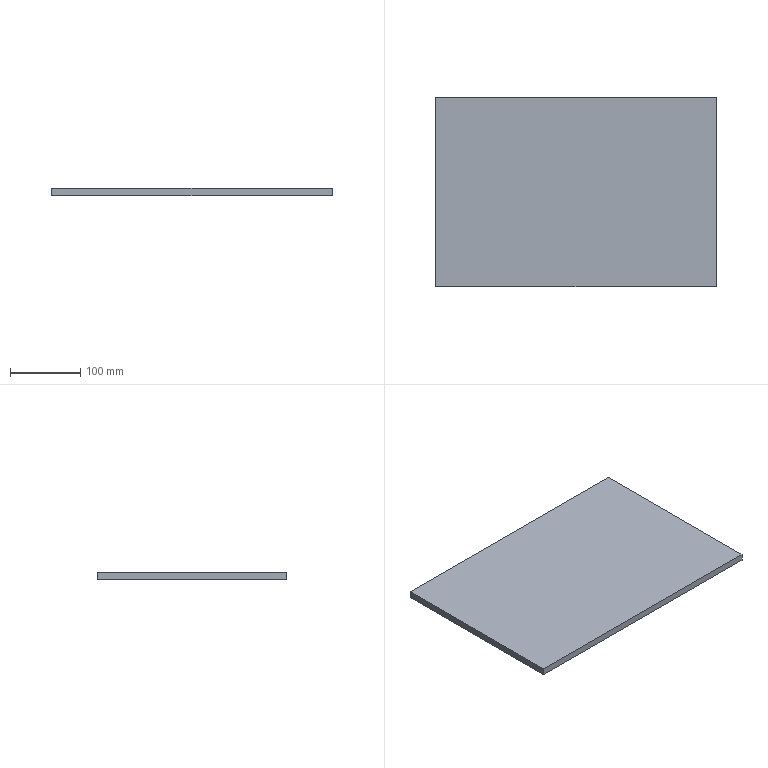Part | SolidWorks | features Extrusion 1 | 1 solid | 6 faces | box 400 x 270 x 10 mm | volume 1080000 mm3 | plane 6
STEP:
#1=CARTESIAN_POINT('',(-200.,135.,-5.));
#2=VERTEX_POINT('',#1);
#3=CARTESIAN_POINT('',(-200.,-135.,-5.));
#4=VERTEX_POINT('',#3);
#5=CARTESIAN_POINT('',(-200.,135.,-5.));
#6=DIRECTION('',(0.,-1.,0.));
#7=VECTOR('',#6,1000.);
#8=LINE('',#5,#7);
#9=EDGE_CURVE('',#2,#4,#8,.T.);
#10=ORIENTED_EDGE('',*,*,#9,.T.);
#11=CARTESIAN_POINT('',(-200.,-135.,5.));
#12=VERTEX_POINT('',#11);
#13=CARTESIAN_POINT('',(-200.,-135.,5.));
#14=DIRECTION('',(0.,0.,-1.));
#15=VECTOR('',#14,1000.);
#16=LINE('',#13,#15);
#17=EDGE_CURVE('',#12,#4,#16,.T.);
#18=ORIENTED_EDGE('',*,*,#17,.F.);
#19=CARTESIAN_POINT('',(-200.,135.,5.));
#20=VERTEX_POINT('',#19);
#21=CARTESIAN_POINT('',(-200.,135.,5.));
#22=DIRECTION('',(0.,-1.,0.));
#23=VECTOR('',#22,1000.);
#24=LINE('',#21,#23);
#25=EDGE_CURVE('',#20,#12,#24,.T.);
#26=ORIENTED_EDGE('',*,*,#25,.F.);
#27=CARTESIAN_POINT('',(-200.,135.,5.));
#28=DIRECTION('',(0.,0.,-1.));
#29=VECTOR('',#28,1000.);
#30=LINE('',#27,#29);
#31=EDGE_CURVE('',#20,#2,#30,.T.);
#32=ORIENTED_EDGE('',*,*,#31,.T.);
#33=EDGE_LOOP('',(#10,#18,#26,#32));
#34=FACE_OUTER_BOUND('',#33,.T.);
#35=CARTESIAN_POINT('',(-200.,135.,5.));
#36=DIRECTION('',(1.,0.,0.));
#37=DIRECTION('',(0.,1.,0.));
#38=AXIS2_PLACEMENT_3D('',#35,#36,#37);
#39=PLANE('',#38);
#40=ADVANCED_FACE('',(#34),#39,.F.);
#41=CARTESIAN_POINT('',(200.,-135.,-5.));
#42=VERTEX_POINT('',#41);
#43=CARTESIAN_POINT('',(-200.,-135.,-5.));
#44=DIRECTION('',(1.,0.,0.));
#45=VECTOR('',#44,1000.);
#46=LINE('',#43,#45);
#47=EDGE_CURVE('',#4,#42,#46,.T.);
#48=ORIENTED_EDGE('',*,*,#47,.T.);
#49=CARTESIAN_POINT('',(200.,-135.,5.));
#50=VERTEX_POINT('',#49);
#51=CARTESIAN_POINT('',(200.,-135.,5.));
#52=DIRECTION('',(0.,0.,-1.));
#53=VECTOR('',#52,1000.);
#54=LINE('',#51,#53);
#55=EDGE_CURVE('',#50,#42,#54,.T.);
#56=ORIENTED_EDGE('',*,*,#55,.F.);
#57=CARTESIAN_POINT('',(-200.,-135.,5.));
#58=DIRECTION('',(1.,0.,0.));
#59=VECTOR('',#58,1000.);
#60=LINE('',#57,#59);
#61=EDGE_CURVE('',#12,#50,#60,.T.);
#62=ORIENTED_EDGE('',*,*,#61,.F.);
#63=ORIENTED_EDGE('',*,*,#17,.T.);
#64=EDGE_LOOP('',(#48,#56,#62,#63));
#65=FACE_OUTER_BOUND('',#64,.T.);
#66=CARTESIAN_POINT('',(-200.,-135.,5.));
#67=DIRECTION('',(0.,1.,0.));
#68=DIRECTION('',(-1.,0.,0.));
#69=AXIS2_PLACEMENT_3D('',#66,#67,#68);
#70=PLANE('',#69);
#71=ADVANCED_FACE('',(#65),#70,.F.);
#72=CARTESIAN_POINT('',(200.,135.,-5.));
#73=VERTEX_POINT('',#72);
#74=CARTESIAN_POINT('',(200.,135.,-5.));
#75=DIRECTION('',(0.,1.,0.));
#76=VECTOR('',#75,1000.);
#77=LINE('',#74,#76);
#78=EDGE_CURVE('',#42,#73,#77,.T.);
#79=ORIENTED_EDGE('',*,*,#78,.T.);
#80=CARTESIAN_POINT('',(200.,135.,5.));
#81=VERTEX_POINT('',#80);
#82=CARTESIAN_POINT('',(200.,135.,5.));
#83=DIRECTION('',(0.,0.,-1.));
#84=VECTOR('',#83,1000.);
#85=LINE('',#82,#84);
#86=EDGE_CURVE('',#81,#73,#85,.T.);
#87=ORIENTED_EDGE('',*,*,#86,.F.);
#88=CARTESIAN_POINT('',(200.,135.,5.));
#89=DIRECTION('',(0.,1.,0.));
#90=VECTOR('',#89,1000.);
#91=LINE('',#88,#90);
#92=EDGE_CURVE('',#50,#81,#91,.T.);
#93=ORIENTED_EDGE('',*,*,#92,.F.);
#94=ORIENTED_EDGE('',*,*,#55,.T.);
#95=EDGE_LOOP('',(#79,#87,#93,#94));
#96=FACE_OUTER_BOUND('',#95,.T.);
#97=CARTESIAN_POINT('',(200.,135.,5.));
#98=DIRECTION('',(-1.,0.,0.));
#99=DIRECTION('',(0.,-1.,0.));
#100=AXIS2_PLACEMENT_3D('',#97,#98,#99);
#101=PLANE('',#100);
#102=ADVANCED_FACE('',(#96),#101,.F.);
#103=CARTESIAN_POINT('',(-200.,135.,-5.));
#104=DIRECTION('',(-1.,0.,0.));
#105=VECTOR('',#104,1000.);
#106=LINE('',#103,#105);
#107=EDGE_CURVE('',#73,#2,#106,.T.);
#108=ORIENTED_EDGE('',*,*,#107,.T.);
#109=ORIENTED_EDGE('',*,*,#31,.F.);
#110=CARTESIAN_POINT('',(-200.,135.,5.));
#111=DIRECTION('',(-1.,0.,0.));
#112=VECTOR('',#111,1000.);
#113=LINE('',#110,#112);
#114=EDGE_CURVE('',#81,#20,#113,.T.);
#115=ORIENTED_EDGE('',*,*,#114,.F.);
#116=ORIENTED_EDGE('',*,*,#86,.T.);
#117=EDGE_LOOP('',(#108,#109,#115,#116));
#118=FACE_OUTER_BOUND('',#117,.T.);
#119=CARTESIAN_POINT('',(-200.,135.,5.));
#120=DIRECTION('',(0.,-1.,0.));
#121=DIRECTION('',(0.,0.,-1.));
#122=AXIS2_PLACEMENT_3D('',#119,#120,#121);
#123=PLANE('',#122);
#124=ADVANCED_FACE('',(#118),#123,.F.);
#125=ORIENTED_EDGE('',*,*,#25,.T.);
#126=ORIENTED_EDGE('',*,*,#61,.T.);
#127=ORIENTED_EDGE('',*,*,#92,.T.);
#128=ORIENTED_EDGE('',*,*,#114,.T.);
#129=EDGE_LOOP('',(#125,#126,#127,#128));
#130=FACE_OUTER_BOUND('',#129,.T.);
#131=CARTESIAN_POINT('',(-200.,-135.,5.));
#132=DIRECTION('',(0.,0.,1.));
#133=DIRECTION('',(1.,0.,0.));
#134=AXIS2_PLACEMENT_3D('',#131,#132,#133);
#135=PLANE('',#134);
#136=ADVANCED_FACE('',(#130),#135,.T.);
#137=ORIENTED_EDGE('',*,*,#9,.F.);
#138=ORIENTED_EDGE('',*,*,#107,.F.);
#139=ORIENTED_EDGE('',*,*,#78,.F.);
#140=ORIENTED_EDGE('',*,*,#47,.F.);
#141=EDGE_LOOP('',(#137,#138,#139,#140));
#142=FACE_OUTER_BOUND('',#141,.T.);
#143=CARTESIAN_POINT('',(-200.,-135.,-5.));
#144=DIRECTION('',(0.,0.,1.));
#145=DIRECTION('',(1.,0.,0.));
#146=AXIS2_PLACEMENT_3D('',#143,#144,#145);
#147=PLANE('',#146);
#148=ADVANCED_FACE('',(#142),#147,.F.);
#149=CLOSED_SHELL('',(#40,#71,#102,#124,#136,#148));
#150=MANIFOLD_SOLID_BREP('',#149);
#151=CARTESIAN_POINT('',(0.,0.,0.));
#152=DIRECTION('',(0.,0.,1.));
#153=DIRECTION('',(1.,0.,0.));
#154=AXIS2_PLACEMENT_3D('',#151,#152,#153);
#155=(LENGTH_UNIT()NAMED_UNIT(*)SI_UNIT(.MILLI.,.METRE.));
#156=UNCERTAINTY_MEASURE_WITH_UNIT(LENGTH_MEASURE(0.00001),#155,'','');
#157=(NAMED_UNIT(*)PLANE_ANGLE_UNIT()SI_UNIT($,.RADIAN.));
#158=(NAMED_UNIT(*)SI_UNIT($,.STERADIAN.)SOLID_ANGLE_UNIT());
#159=(GEOMETRIC_REPRESENTATION_CONTEXT(3)GLOBAL_UNCERTAINTY_ASSIGNED_CONTEXT((#156))GLOBAL_UNIT_ASSIGNED_CONTEXT((#155,#157,#158))REPRESENTATION_CONTEXT('',''));
#160=ADVANCED_BREP_SHAPE_REPRESENTATION('',(#150,#154),#159);